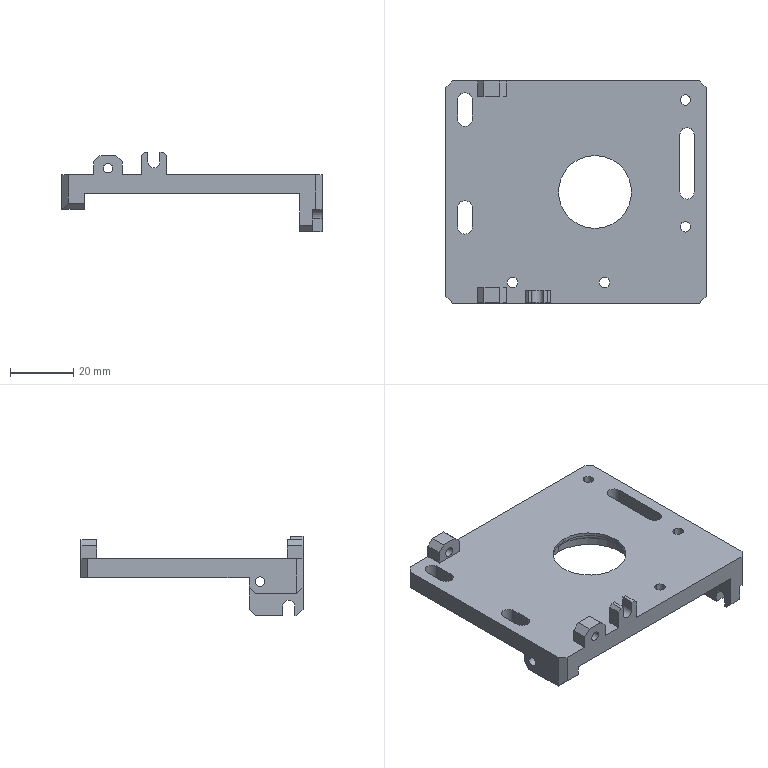NC program | NX | posted with a generic post | part box 82 x 70 x 25 mm
Lines 1409 to 2271 of 8354:
(ZLEVEL_PROFILE_1_1 , TOOL : D3)
N2792 T03 M6
N2794 G54
N2796 G17 G0 G90 X6.477 Y34.25 S9500 M3
N2798 G43 Z30. H3
N2800 Z-11.
N2802 G94 G1 X18.123 Z-11.61 F1000.
N2804 X18.342 Y34.321 Z-11.622
N2806 X18.541 Y34.466 Z-11.635
N2808 X18.704 Y34.713 Z-11.651
N2810 X18.76 Y35.005 Z-11.666
N2812 X18.7 Y35.295 Z-11.682
N2814 X18.534 Y35.541 Z-11.697
N2816 X18.333 Y35.683 Z-11.71
N2818 X18.123 Y35.75 Z-11.722
N2820 X9.001 Z-12.2
N2822 X0.001 F1300.
N2824 G3 X-0.75 Y35.008 R0.75
N2826 X0.007 Y34.25 R0.75
N2828 G1 X18.
N2830 G3 X18.75 Y35. R0.75
N2832 X18. Y35.75 R0.75
N2834 G1 X9.001
N2836 X0.224 Z-12.353
N2838 X0.102 Z-12.355
N2840 X-0.019 Y35.744 Z-12.357
N2842 X-0.186 Y35.718 Z-12.36
N2844 X-0.256 Y35.699 Z-12.362
N2846 X-0.381 Y35.639 Z-12.364
N2848 X-0.466 Y35.581 Z-12.366
N2850 X-0.532 Y35.517 Z-12.368
N2852 X-0.565 Y35.486
N2854 X-0.587 Y35.458 Z-12.369
N2856 X-0.625 Y35.4 Z-12.37
N2858 X-0.675 Y35.309 Z-12.372
N2860 X-0.697 Y35.263 Z-12.373
N2862 X-0.706 Y35.236
N2864 X-0.72 Y35.18 Z-12.374
N2866 X-0.743 Y35.02 Z-12.377
N2868 X-0.74 Y34.94 Z-12.379
N2870 X-0.714 Y34.797 Z-12.381
N2872 X-0.682 Y34.707 Z-12.383
N2874 X-0.611 Y34.58 Z-12.386
N2876 X-0.554 Y34.503 Z-12.387
N2878 X-0.458 Y34.414 Z-12.39
N2880 X-0.367 Y34.352 Z-12.391
N2882 X-0.236 Y34.288 Z-12.394
N2884 X-0.205 Y34.279 Z-12.395
N2886 X-0.142 Y34.264 Z-12.396
N2888 X-0.02 Y34.256 Z-12.398
N2890 X0.101 Y34.25 Z-12.4
N2892 X18.
N2894 G3 X18.75 Y35. R0.75
N2896 X18. Y35.75 R0.75
N2898 G1 X9.001
N2900 X0.224 Z-12.553
N2902 X0.102 Z-12.555
N2904 X-0.019 Y35.744 Z-12.557
N2906 X-0.186 Y35.718 Z-12.56
N2908 X-0.256 Y35.699 Z-12.562
N2910 X-0.381 Y35.639 Z-12.564
N2912 X-0.466 Y35.581 Z-12.566
N2914 X-0.532 Y35.517 Z-12.568
N2916 X-0.565 Y35.486
N2918 X-0.587 Y35.458 Z-12.569
N2920 X-0.625 Y35.4 Z-12.57
N2922 X-0.675 Y35.309 Z-12.572
N2924 X-0.697 Y35.263 Z-12.573
N2926 X-0.706 Y35.236
N2928 X-0.72 Y35.18 Z-12.574
N2930 X-0.743 Y35.02 Z-12.577
N2932 X-0.74 Y34.94 Z-12.579
N2934 X-0.714 Y34.797 Z-12.581
N2936 X-0.682 Y34.707 Z-12.583
N2938 X-0.611 Y34.58 Z-12.586
N2940 X-0.554 Y34.503 Z-12.587
N2942 X-0.458 Y34.414 Z-12.59
N2944 X-0.367 Y34.352 Z-12.591
N2946 X-0.236 Y34.288 Z-12.594
N2948 X-0.205 Y34.279 Z-12.595
N2950 X-0.142 Y34.264 Z-12.596
N2952 X-0.02 Y34.256 Z-12.598
N2954 X0.101 Y34.25 Z-12.6
N2956 X18.
N2958 G3 X18.75 Y35. R0.75
N2960 X18. Y35.75 R0.75
N2962 G1 X9.001
N2964 X0.224 Z-12.753
N2966 X0.102 Z-12.755
N2968 X-0.019 Y35.744 Z-12.757
N2970 X-0.186 Y35.718 Z-12.76
N2972 X-0.256 Y35.699 Z-12.762
N2974 X-0.381 Y35.639 Z-12.764
N2976 X-0.466 Y35.581 Z-12.766
N2978 X-0.532 Y35.517 Z-12.768
N2980 X-0.565 Y35.486
N2982 X-0.587 Y35.458 Z-12.769
N2984 X-0.625 Y35.4 Z-12.77
N2986 X-0.675 Y35.309 Z-12.772
N2988 X-0.697 Y35.263 Z-12.773
N2990 X-0.706 Y35.236
N2992 X-0.72 Y35.18 Z-12.774
N2994 X-0.743 Y35.02 Z-12.777
N2996 X-0.74 Y34.94 Z-12.779
N2998 X-0.714 Y34.797 Z-12.781
N3000 X-0.682 Y34.707 Z-12.783
N3002 X-0.611 Y34.58 Z-12.786
N3004 X-0.554 Y34.503 Z-12.787
N3006 X-0.458 Y34.414 Z-12.79
N3008 X-0.367 Y34.352 Z-12.791
N3010 X-0.236 Y34.288 Z-12.794
N3012 X-0.205 Y34.279 Z-12.795
N3014 X-0.142 Y34.264 Z-12.796
N3016 X-0.02 Y34.256 Z-12.798
N3018 X0.101 Y34.25 Z-12.8
N3020 X18.
N3022 G3 X18.75 Y35. R0.75
N3024 X18. Y35.75 R0.75
N3026 G1 X9.001
N3028 X0.224 Z-12.953
N3030 X0.102 Z-12.955
N3032 X-0.019 Y35.744 Z-12.957
N3034 X-0.186 Y35.718 Z-12.96
N3036 X-0.256 Y35.699 Z-12.962
N3038 X-0.381 Y35.639 Z-12.964
N3040 X-0.466 Y35.581 Z-12.966
N3042 X-0.532 Y35.517 Z-12.968
N3044 X-0.565 Y35.486
N3046 X-0.587 Y35.458 Z-12.969
N3048 X-0.625 Y35.4 Z-12.97
N3050 X-0.675 Y35.31 Z-12.972
N3052 X-0.697 Y35.263 Z-12.973
N3054 X-0.706 Y35.236
N3056 X-0.72 Y35.18 Z-12.974
N3058 X-0.743 Y35.021 Z-12.977
N3060 X-0.74 Y34.94 Z-12.979
N3062 X-0.714 Y34.797 Z-12.981
N3064 X-0.682 Y34.707 Z-12.983
N3066 X-0.611 Y34.58 Z-12.986
N3068 X-0.554 Y34.503 Z-12.987
N3070 X-0.458 Y34.414 Z-12.99
N3072 X-0.367 Y34.352 Z-12.991
N3074 X-0.236 Y34.288 Z-12.994
N3076 X-0.205 Y34.279 Z-12.995
N3078 X-0.142 Y34.264 Z-12.996
N3080 X-0.02 Y34.256 Z-12.998
N3082 X0.101 Y34.25 Z-13.
N3084 X18.
N3086 G3 X18.75 Y35. R0.75
N3088 X18. Y35.75 R0.75
N3090 G1 X9.001
N3092 X0.224 Z-13.153
N3094 X0.102 Z-13.155
N3096 X-0.019 Y35.744 Z-13.157
N3098 X-0.186 Y35.718 Z-13.16
N3100 X-0.256 Y35.699 Z-13.162
N3102 X-0.381 Y35.639 Z-13.164
N3104 X-0.466 Y35.581 Z-13.166
N3106 X-0.532 Y35.517 Z-13.168
N3108 X-0.565 Y35.486
N3110 X-0.587 Y35.458 Z-13.169
N3112 X-0.625 Y35.4 Z-13.17
N3114 X-0.675 Y35.31 Z-13.172
N3116 X-0.697 Y35.263 Z-13.173
N3118 X-0.706 Y35.236
N3120 X-0.72 Y35.18 Z-13.174
N3122 X-0.743 Y35.021 Z-13.177
N3124 X-0.74 Y34.94 Z-13.179
N3126 X-0.714 Y34.797 Z-13.181
N3128 X-0.682 Y34.707 Z-13.183
N3130 X-0.611 Y34.58 Z-13.186
N3132 X-0.554 Y34.503 Z-13.187
N3134 X-0.458 Y34.414 Z-13.19
N3136 X-0.367 Y34.352 Z-13.191
N3138 X-0.236 Y34.288 Z-13.194
N3140 X-0.205 Y34.279 Z-13.195
N3142 X-0.142 Y34.264 Z-13.196
N3144 X-0.02 Y34.256 Z-13.198
N3146 X0.101 Y34.25 Z-13.2
N3148 X18.
N3150 G3 X18.75 Y35. R0.75
N3152 X18. Y35.75 R0.75
N3154 G1 X9.001
N3156 X0.224 Z-13.353
N3158 X0.102 Z-13.355
N3160 X-0.019 Y35.744 Z-13.357
N3162 X-0.186 Y35.718 Z-13.36
N3164 X-0.256 Y35.699 Z-13.362
N3166 X-0.381 Y35.639 Z-13.364
N3168 X-0.466 Y35.581 Z-13.366
N3170 X-0.532 Y35.517 Z-13.368
N3172 X-0.565 Y35.486
N3174 X-0.587 Y35.458 Z-13.369
N3176 X-0.625 Y35.4 Z-13.37
N3178 X-0.675 Y35.31 Z-13.372
N3180 X-0.697 Y35.263 Z-13.373
N3182 X-0.706 Y35.236
N3184 X-0.72 Y35.18 Z-13.374
N3186 X-0.743 Y35.021 Z-13.377
N3188 X-0.74 Y34.94 Z-13.379
N3190 X-0.714 Y34.797 Z-13.381
N3192 X-0.682 Y34.707 Z-13.383
N3194 X-0.611 Y34.58 Z-13.386
N3196 X-0.554 Y34.503 Z-13.387
N3198 X-0.458 Y34.414 Z-13.39
N3200 X-0.367 Y34.352 Z-13.391
N3202 X-0.236 Y34.288 Z-13.394
N3204 X-0.205 Y34.279 Z-13.395
N3206 X-0.142 Y34.264 Z-13.396
N3208 X-0.02 Y34.256 Z-13.398
N3210 X0.101 Y34.25 Z-13.4
N3212 X18.
N3214 G3 X18.75 Y35. R0.75
N3216 X18. Y35.75 R0.75
N3218 G1 X9.001
N3220 X0.224 Z-13.553
N3222 X0.102 Z-13.555
N3224 X-0.019 Y35.744 Z-13.557
N3226 X-0.186 Y35.718 Z-13.56
N3228 X-0.256 Y35.699 Z-13.562
N3230 X-0.381 Y35.639 Z-13.564
N3232 X-0.466 Y35.581 Z-13.566
N3234 X-0.532 Y35.517 Z-13.568
N3236 X-0.565 Y35.486
N3238 X-0.587 Y35.458 Z-13.569
N3240 X-0.625 Y35.4 Z-13.57
N3242 X-0.675 Y35.31 Z-13.572
N3244 X-0.697 Y35.263 Z-13.573
N3246 X-0.706 Y35.236
N3248 X-0.72 Y35.18 Z-13.574
N3250 X-0.743 Y35.021 Z-13.577
N3252 X-0.74 Y34.94 Z-13.579
N3254 X-0.714 Y34.797 Z-13.581
N3256 X-0.682 Y34.707 Z-13.583
N3258 X-0.611 Y34.58 Z-13.586
N3260 X-0.554 Y34.503 Z-13.587
N3262 X-0.458 Y34.414 Z-13.59
N3264 X-0.367 Y34.352 Z-13.591
N3266 X-0.236 Y34.288 Z-13.594
N3268 X-0.205 Y34.279 Z-13.595
N3270 X-0.142 Y34.264 Z-13.596
N3272 X-0.02 Y34.256 Z-13.598
N3274 X0.101 Y34.25 Z-13.6
N3276 X18.
N3278 G3 X18.75 Y35. R0.75
N3280 X18. Y35.75 R0.75
N3282 G1 X9.001
N3284 X0.224 Z-13.753
N3286 X0.102 Z-13.755
N3288 X-0.019 Y35.744 Z-13.757
N3290 X-0.186 Y35.718 Z-13.76
N3292 X-0.256 Y35.699 Z-13.762
N3294 X-0.381 Y35.639 Z-13.764
N3296 X-0.466 Y35.581 Z-13.766
N3298 X-0.532 Y35.517 Z-13.768
N3300 X-0.565 Y35.486
N3302 X-0.587 Y35.458 Z-13.769
N3304 X-0.625 Y35.4 Z-13.77
N3306 X-0.675 Y35.31 Z-13.772
N3308 X-0.697 Y35.263 Z-13.773
N3310 X-0.706 Y35.236
N3312 X-0.72 Y35.18 Z-13.774
N3314 X-0.743 Y35.021 Z-13.777
N3316 X-0.74 Y34.94 Z-13.779
N3318 X-0.714 Y34.797 Z-13.781
N3320 X-0.682 Y34.707 Z-13.783
N3322 X-0.611 Y34.58 Z-13.786
N3324 X-0.554 Y34.503 Z-13.787
N3326 X-0.458 Y34.414 Z-13.79
N3328 X-0.367 Y34.352 Z-13.791
N3330 X-0.236 Y34.288 Z-13.794
N3332 X-0.205 Y34.279 Z-13.795
N3334 X-0.142 Y34.264 Z-13.796
N3336 X-0.02 Y34.256 Z-13.798
N3338 X0.101 Y34.25 Z-13.8
N3340 X18.
N3342 G3 X18.75 Y35. R0.75
N3344 X18. Y35.75 R0.75
N3346 G1 X9.001
N3348 X0.224 Z-13.953
N3350 X0.102 Z-13.955
N3352 X-0.019 Y35.744 Z-13.957
N3354 X-0.186 Y35.718 Z-13.96
N3356 X-0.256 Y35.699 Z-13.962
N3358 X-0.381 Y35.639 Z-13.964
N3360 X-0.466 Y35.581 Z-13.966
N3362 X-0.532 Y35.517 Z-13.968
N3364 X-0.565 Y35.486
N3366 X-0.587 Y35.458 Z-13.969
N3368 X-0.625 Y35.4 Z-13.97
N3370 X-0.675 Y35.31 Z-13.972
N3372 X-0.697 Y35.263 Z-13.973
N3374 X-0.706 Y35.236
N3376 X-0.72 Y35.18 Z-13.974
N3378 X-0.743 Y35.021 Z-13.977
N3380 X-0.74 Y34.94 Z-13.979
N3382 X-0.714 Y34.797 Z-13.981
N3384 X-0.682 Y34.707 Z-13.983
N3386 X-0.611 Y34.58 Z-13.986
N3388 X-0.554 Y34.503 Z-13.987
N3390 X-0.458 Y34.414 Z-13.99
N3392 X-0.367 Y34.352 Z-13.991
N3394 X-0.236 Y34.288 Z-13.994
N3396 X-0.205 Y34.279 Z-13.995
N3398 X-0.142 Y34.264 Z-13.996
N3400 X-0.02 Y34.256 Z-13.998
N3402 X0.101 Y34.25 Z-14.
N3404 X18.
N3406 G3 X18.75 Y35. R0.75
N3408 X18. Y35.75 R0.75
N3410 G1 X9.001
N3412 X0.224 Z-14.153
N3414 X0.102 Z-14.155
N3416 X-0.019 Y35.744 Z-14.157
N3418 X-0.186 Y35.718 Z-14.16
N3420 X-0.256 Y35.699 Z-14.162
N3422 X-0.381 Y35.639 Z-14.164
N3424 X-0.466 Y35.581 Z-14.166
N3426 X-0.532 Y35.517 Z-14.168
N3428 X-0.565 Y35.486
N3430 X-0.586 Y35.458 Z-14.169
N3432 X-0.625 Y35.4 Z-14.17
N3434 X-0.675 Y35.31 Z-14.172
N3436 X-0.697 Y35.263 Z-14.173
N3438 X-0.706 Y35.236
N3440 X-0.72 Y35.18 Z-14.174
N3442 X-0.743 Y35.021 Z-14.177
N3444 X-0.74 Y34.94 Z-14.179
N3446 X-0.714 Y34.797 Z-14.181
N3448 X-0.682 Y34.707 Z-14.183
N3450 X-0.611 Y34.58 Z-14.186
N3452 X-0.554 Y34.503 Z-14.187
N3454 X-0.458 Y34.414 Z-14.19
N3456 X-0.367 Y34.352 Z-14.191
N3458 X-0.236 Y34.288 Z-14.194
N3460 X-0.205 Y34.279 Z-14.195
N3462 X-0.142 Y34.264 Z-14.196
N3464 X-0.02 Y34.256 Z-14.198
N3466 X0.101 Y34.25 Z-14.2
N3468 X18.
N3470 G3 X18.75 Y35. R0.75
N3472 X18. Y35.75 R0.75
N3474 G1 X9.001
N3476 X0.224 Z-14.353
N3478 X0.102 Z-14.355
N3480 X-0.019 Y35.744 Z-14.357
N3482 X-0.186 Y35.718 Z-14.36
N3484 X-0.256 Y35.699 Z-14.362
N3486 X-0.381 Y35.639 Z-14.364
N3488 X-0.466 Y35.581 Z-14.366
N3490 X-0.532 Y35.517 Z-14.368
N3492 X-0.565 Y35.486
N3494 X-0.586 Y35.458 Z-14.369
N3496 X-0.625 Y35.4 Z-14.37
N3498 X-0.675 Y35.31 Z-14.372
N3500 X-0.697 Y35.263 Z-14.373
N3502 X-0.706 Y35.236
N3504 X-0.72 Y35.18 Z-14.374
N3506 X-0.743 Y35.021 Z-14.377
N3508 X-0.74 Y34.94 Z-14.379
N3510 X-0.714 Y34.797 Z-14.381
N3512 X-0.682 Y34.707 Z-14.383
N3514 X-0.611 Y34.58 Z-14.386
N3516 X-0.554 Y34.503 Z-14.387
N3518 X-0.458 Y34.414 Z-14.39
N3520 X-0.367 Y34.352 Z-14.391
N3522 X-0.236 Y34.288 Z-14.394
N3524 X-0.205 Y34.279 Z-14.395
N3526 X-0.142 Y34.264 Z-14.396
N3528 X-0.02 Y34.256 Z-14.398
N3530 X0.101 Y34.25 Z-14.4
N3532 X18.
N3534 G3 X18.75 Y35. R0.75
N3536 X18. Y35.75 R0.75
N3538 G1 X9.001
N3540 X0.224 Z-14.553
N3542 X0.102 Z-14.555
N3544 X-0.019 Y35.744 Z-14.557
N3546 X-0.186 Y35.718 Z-14.56
N3548 X-0.256 Y35.699 Z-14.562
N3550 X-0.381 Y35.639 Z-14.564
N3552 X-0.466 Y35.581 Z-14.566
N3554 X-0.532 Y35.517 Z-14.568
N3556 X-0.565 Y35.486
N3558 X-0.586 Y35.458 Z-14.569
N3560 X-0.625 Y35.4 Z-14.57
N3562 X-0.675 Y35.31 Z-14.572
N3564 X-0.697 Y35.263 Z-14.573
N3566 X-0.706 Y35.236
N3568 X-0.72 Y35.18 Z-14.574
N3570 X-0.743 Y35.021 Z-14.577
N3572 X-0.74 Y34.94 Z-14.579
N3574 X-0.714 Y34.797 Z-14.581
N3576 X-0.682 Y34.707 Z-14.583
N3578 X-0.611 Y34.58 Z-14.586
N3580 X-0.554 Y34.503 Z-14.587
N3582 X-0.458 Y34.414 Z-14.59
N3584 X-0.367 Y34.352 Z-14.591
N3586 X-0.236 Y34.288 Z-14.594
N3588 X-0.205 Y34.279 Z-14.595
N3590 X-0.142 Y34.264 Z-14.596
N3592 X-0.02 Y34.256 Z-14.598
N3594 X0.101 Y34.25 Z-14.6
N3596 X18.
N3598 G3 X18.75 Y35. R0.75
N3600 X18. Y35.75 R0.75
N3602 G1 X9.001
N3604 X0.224 Z-14.753
N3606 X0.102 Z-14.755
N3608 X-0.019 Y35.744 Z-14.757
N3610 X-0.186 Y35.718 Z-14.76
N3612 X-0.256 Y35.699 Z-14.762
N3614 X-0.381 Y35.639 Z-14.764
N3616 X-0.466 Y35.581 Z-14.766
N3618 X-0.532 Y35.517 Z-14.768
N3620 X-0.565 Y35.486
N3622 X-0.586 Y35.458 Z-14.769
N3624 X-0.625 Y35.4 Z-14.77
N3626 X-0.675 Y35.31 Z-14.772
N3628 X-0.697 Y35.263 Z-14.773
N3630 X-0.706 Y35.236
N3632 X-0.72 Y35.18 Z-14.774
N3634 X-0.743 Y35.021 Z-14.777
N3636 X-0.74 Y34.94 Z-14.779
N3638 X-0.714 Y34.797 Z-14.781
N3640 X-0.682 Y34.707 Z-14.783
N3642 X-0.611 Y34.58 Z-14.786
N3644 X-0.554 Y34.503 Z-14.787
N3646 X-0.458 Y34.414 Z-14.79
N3648 X-0.367 Y34.352 Z-14.791
N3650 X-0.236 Y34.288 Z-14.794
N3652 X-0.205 Y34.279 Z-14.795
N3654 X-0.142 Y34.264 Z-14.796
N3656 X-0.02 Y34.256 Z-14.798
N3658 X0.101 Y34.25 Z-14.8
N3660 X18.
N3662 G3 X18.75 Y35. R0.75
N3664 X18. Y35.75 R0.75
N3666 G1 X9.001
N3668 X0.224 Z-14.953
N3670 X0.102 Z-14.955
N3672 X-0.019 Y35.744 Z-14.957
N3674 X-0.186 Y35.718 Z-14.96
N3676 X-0.256 Y35.699 Z-14.962
N3678 X-0.381 Y35.639 Z-14.964
N3680 X-0.466 Y35.581 Z-14.966
N3682 X-0.532 Y35.517 Z-14.968
N3684 X-0.565 Y35.486
N3686 X-0.586 Y35.458 Z-14.969
N3688 X-0.625 Y35.4 Z-14.97
N3690 X-0.675 Y35.31 Z-14.972
N3692 X-0.697 Y35.263 Z-14.973
N3694 X-0.706 Y35.236
N3696 X-0.72 Y35.18 Z-14.974
N3698 X-0.743 Y35.021 Z-14.977
N3700 X-0.74 Y34.94 Z-14.979
N3702 X-0.714 Y34.797 Z-14.981
N3704 X-0.682 Y34.707 Z-14.983
N3706 X-0.611 Y34.58 Z-14.986
N3708 X-0.554 Y34.503 Z-14.987
N3710 X-0.458 Y34.414 Z-14.99
N3712 X-0.367 Y34.352 Z-14.991
N3714 X-0.236 Y34.288 Z-14.994
N3716 X-0.205 Y34.279 Z-14.995
N3718 X-0.142 Y34.264 Z-14.996
N3720 X-0.02 Y34.256 Z-14.998
N3722 X0.101 Y34.25 Z-15.
N3724 X18.
N3726 G3 X18.75 Y35. R0.75
N3728 X18. Y35.75 R0.75
N3730 G1 X9.001
N3732 X0.224 Z-15.153
N3734 X0.102 Z-15.155
N3736 X-0.019 Y35.744 Z-15.157
N3738 X-0.186 Y35.718 Z-15.16
N3740 X-0.256 Y35.699 Z-15.162
N3742 X-0.381 Y35.639 Z-15.164
N3744 X-0.466 Y35.581 Z-15.166
N3746 X-0.532 Y35.517 Z-15.168
N3748 X-0.565 Y35.486
N3750 X-0.586 Y35.458 Z-15.169
N3752 X-0.625 Y35.4 Z-15.17
N3754 X-0.675 Y35.31 Z-15.172
N3756 X-0.697 Y35.263 Z-15.173
N3758 X-0.706 Y35.236
N3760 X-0.72 Y35.18 Z-15.174
N3762 X-0.743 Y35.021 Z-15.177
N3764 X-0.74 Y34.94 Z-15.179
N3766 X-0.714 Y34.797 Z-15.181
N3768 X-0.682 Y34.707 Z-15.183
N3770 X-0.611 Y34.58 Z-15.186
N3772 X-0.554 Y34.503 Z-15.187
N3774 X-0.458 Y34.414 Z-15.19
N3776 X-0.367 Y34.352 Z-15.191
N3778 X-0.236 Y34.288 Z-15.194
N3780 X-0.205 Y34.279 Z-15.195
N3782 X-0.142 Y34.264 Z-15.196
N3784 X-0.02 Y34.256 Z-15.198
N3786 X0.101 Y34.25 Z-15.2
N3788 X18.
N3790 G3 X18.75 Y35. R0.75
N3792 X18. Y35.75 R0.75
N3794 G1 X9.001
N3796 X0.224 Z-15.353
N3798 X0.102 Z-15.355
N3800 X-0.019 Y35.744 Z-15.357
N3802 X-0.186 Y35.718 Z-15.36
N3804 X-0.256 Y35.699 Z-15.362
N3806 X-0.381 Y35.639 Z-15.364
N3808 X-0.466 Y35.581 Z-15.366
N3810 X-0.532 Y35.517 Z-15.368
N3812 X-0.565 Y35.486
N3814 X-0.586 Y35.458 Z-15.369
N3816 X-0.625 Y35.4 Z-15.37
N3818 X-0.675 Y35.31 Z-15.372
N3820 X-0.697 Y35.263 Z-15.373
N3822 X-0.706 Y35.236
N3824 X-0.72 Y35.18 Z-15.374
N3826 X-0.743 Y35.021 Z-15.377
N3828 X-0.74 Y34.94 Z-15.379
N3830 X-0.714 Y34.797 Z-15.381
N3832 X-0.682 Y34.707 Z-15.383
N3834 X-0.611 Y34.58 Z-15.386
N3836 X-0.554 Y34.503 Z-15.387
N3838 X-0.458 Y34.414 Z-15.39
N3840 X-0.367 Y34.352 Z-15.391
N3842 X-0.236 Y34.288 Z-15.394
N3844 X-0.205 Y34.279 Z-15.395
N3846 X-0.142 Y34.264 Z-15.396
N3848 X-0.02 Y34.256 Z-15.398
N3850 X0.101 Y34.25 Z-15.4
N3852 X18.
N3854 G3 X18.75 Y35. R0.75
N3856 X18. Y35.75 R0.75
N3858 G1 X9.001
N3860 X0.224 Z-15.553
N3862 X0.102 Z-15.555
N3864 X-0.019 Y35.744 Z-15.557
N3866 X-0.186 Y35.718 Z-15.56
N3868 X-0.256 Y35.699 Z-15.562
N3870 X-0.381 Y35.639 Z-15.564
N3872 X-0.466 Y35.581 Z-15.566
N3874 X-0.532 Y35.517 Z-15.568
N3876 X-0.565 Y35.486
N3878 X-0.586 Y35.458 Z-15.569
N3880 X-0.625 Y35.4 Z-15.57
N3882 X-0.675 Y35.31 Z-15.572
N3884 X-0.697 Y35.263 Z-15.573
N3886 X-0.706 Y35.236
N3888 X-0.72 Y35.18 Z-15.574
N3890 X-0.743 Y35.021 Z-15.577
N3892 X-0.74 Y34.94 Z-15.579
N3894 X-0.714 Y34.797 Z-15.581
N3896 X-0.682 Y34.707 Z-15.583
N3898 X-0.611 Y34.58 Z-15.586
N3900 X-0.554 Y34.503 Z-15.587
N3902 X-0.458 Y34.414 Z-15.59
N3904 X-0.367 Y34.352 Z-15.591
N3906 X-0.236 Y34.288 Z-15.594
N3908 X-0.205 Y34.279 Z-15.595
N3910 X-0.142 Y34.264 Z-15.596
N3912 X-0.02 Y34.256 Z-15.598
N3914 X0.101 Y34.25 Z-15.6
N3916 X18.
N3918 G3 X18.75 Y35. R0.75
N3920 X18. Y35.75 R0.75
N3922 G1 X9.001
N3924 X0.224 Z-15.753
N3926 X0.102 Z-15.755
N3928 X-0.019 Y35.744 Z-15.757
N3930 X-0.186 Y35.718 Z-15.76
N3932 X-0.256 Y35.699 Z-15.762
N3934 X-0.381 Y35.639 Z-15.764
N3936 X-0.466 Y35.581 Z-15.766
N3938 X-0.532 Y35.517 Z-15.768
N3940 X-0.565 Y35.486
N3942 X-0.586 Y35.458 Z-15.769
N3944 X-0.625 Y35.4 Z-15.77
N3946 X-0.675 Y35.31 Z-15.772
N3948 X-0.697 Y35.263 Z-15.773
N3950 X-0.706 Y35.236
N3952 X-0.72 Y35.18 Z-15.774
N3954 X-0.743 Y35.021 Z-15.777
N3956 X-0.74 Y34.94 Z-15.779
N3958 X-0.714 Y34.797 Z-15.781
N3960 X-0.682 Y34.707 Z-15.783
N3962 X-0.611 Y34.58 Z-15.786
N3964 X-0.554 Y34.503 Z-15.787
N3966 X-0.458 Y34.414 Z-15.79
N3968 X-0.367 Y34.352 Z-15.791
N3970 X-0.236 Y34.288 Z-15.794
N3972 X-0.205 Y34.279 Z-15.795
N3974 X-0.142 Y34.264 Z-15.796
N3976 X-0.02 Y34.256 Z-15.798
N3978 X0.101 Y34.25 Z-15.8
N3980 X18.
N3982 G3 X18.75 Y35. R0.75
N3984 X18. Y35.75 R0.75
N3986 G1 X9.001
N3988 X0.224 Z-15.953
N3990 X0.102 Z-15.955
N3992 X-0.019 Y35.744 Z-15.957
N3994 X-0.186 Y35.718 Z-15.96
N3996 X-0.256 Y35.699 Z-15.962
N3998 X-0.381 Y35.639 Z-15.964
N4000 X-0.466 Y35.581 Z-15.966
N4002 X-0.532 Y35.517 Z-15.968
N4004 X-0.565 Y35.486
N4006 X-0.586 Y35.458 Z-15.969
N4008 X-0.625 Y35.4 Z-15.97
N4010 X-0.675 Y35.31 Z-15.972
N4012 X-0.697 Y35.263 Z-15.973
N4014 X-0.706 Y35.236
N4016 X-0.72 Y35.18 Z-15.974
N4018 X-0.743 Y35.021 Z-15.977
N4020 X-0.74 Y34.94 Z-15.979
N4022 X-0.714 Y34.797 Z-15.981
N4024 X-0.682 Y34.707 Z-15.983
N4026 X-0.611 Y34.58 Z-15.986
N4028 X-0.554 Y34.503 Z-15.987
N4030 X-0.458 Y34.414 Z-15.99
N4032 X-0.367 Y34.352 Z-15.991
N4034 X-0.236 Y34.288 Z-15.994
N4036 X-0.205 Y34.279 Z-15.995
N4038 X-0.142 Y34.264 Z-15.996
N4040 X-0.02 Y34.256 Z-15.998
N4042 X0.101 Y34.25 Z-16.
N4044 X18.
N4046 G3 X18.75 Y35. R0.75
N4048 X18. Y35.75 R0.75
N4050 G1 X9.001
N4052 X0.224 Z-16.153
N4054 X0.102 Z-16.155
N4056 X-0.019 Y35.744 Z-16.157
N4058 X-0.186 Y35.718 Z-16.16
N4060 X-0.256 Y35.699 Z-16.162
N4062 X-0.381 Y35.639 Z-16.164
N4064 X-0.466 Y35.581 Z-16.166
N4066 X-0.532 Y35.517 Z-16.168
N4068 X-0.565 Y35.486
N4070 X-0.586 Y35.458 Z-16.169
N4072 X-0.625 Y35.4 Z-16.17
N4074 X-0.675 Y35.31 Z-16.172
N4076 X-0.697 Y35.263 Z-16.173
N4078 X-0.706 Y35.236
N4080 X-0.72 Y35.18 Z-16.174
N4082 X-0.743 Y35.021 Z-16.177
N4084 X-0.74 Y34.94 Z-16.179
N4086 X-0.714 Y34.797 Z-16.181
N4088 X-0.682 Y34.707 Z-16.183
N4090 X-0.611 Y34.58 Z-16.186
N4092 X-0.554 Y34.503 Z-16.187
N4094 X-0.458 Y34.414 Z-16.19
N4096 X-0.367 Y34.352 Z-16.191
N4098 X-0.236 Y34.288 Z-16.194
N4100 X-0.205 Y34.279 Z-16.195
N4102 X-0.142 Y34.264 Z-16.196
N4104 X-0.02 Y34.256 Z-16.198
N4106 X0.101 Y34.25 Z-16.2
N4108 X18.
N4110 G3 X18.75 Y35. R0.75
N4112 X18. Y35.75 R0.75
N4114 G1 X9.001
N4116 X0.224 Z-16.353
N4118 X0.102 Z-16.355
N4120 X-0.019 Y35.744 Z-16.357
N4122 X-0.186 Y35.718 Z-16.36
N4124 X-0.256 Y35.699 Z-16.362
N4126 X-0.381 Y35.639 Z-16.364
N4128 X-0.466 Y35.581 Z-16.366
N4130 X-0.532 Y35.517 Z-16.368
N4132 X-0.565 Y35.486
N4134 X-0.586 Y35.458 Z-16.369
N4136 X-0.625 Y35.4 Z-16.37
N4138 X-0.675 Y35.31 Z-16.372
N4140 X-0.697 Y35.263 Z-16.373
N4142 X-0.706 Y35.236
N4144 X-0.72 Y35.18 Z-16.374
N4146 X-0.743 Y35.021 Z-16.377
N4148 X-0.74 Y34.94 Z-16.379
N4150 X-0.714 Y34.797 Z-16.381
N4152 X-0.682 Y34.707 Z-16.383
N4154 X-0.611 Y34.58 Z-16.386
N4156 X-0.554 Y34.503 Z-16.387
N4158 X-0.458 Y34.414 Z-16.39
N4160 X-0.367 Y34.352 Z-16.391
N4162 X-0.236 Y34.288 Z-16.394
N4164 X-0.205 Y34.279 Z-16.395
N4166 X-0.142 Y34.264 Z-16.396
N4168 X-0.02 Y34.256 Z-16.398
N4170 X0.101 Y34.25 Z-16.4
N4172 X18.
N4174 G3 X18.75 Y35. R0.75
N4176 X18. Y35.75 R0.75
N4178 G1 X9.001
N4180 X0.224 Z-16.553
N4182 X0.102 Z-16.555
N4184 X-0.019 Y35.744 Z-16.557
N4186 X-0.186 Y35.718 Z-16.56
N4188 X-0.256 Y35.699 Z-16.562
N4190 X-0.381 Y35.639 Z-16.564
N4192 X-0.466 Y35.581 Z-16.566
N4194 X-0.532 Y35.517 Z-16.568
N4196 X-0.565 Y35.486
N4198 X-0.586 Y35.458 Z-16.569
N4200 X-0.625 Y35.4 Z-16.57
N4202 X-0.675 Y35.31 Z-16.572
N4204 X-0.697 Y35.263 Z-16.573
N4206 X-0.706 Y35.236
N4208 X-0.72 Y35.18 Z-16.574
N4210 X-0.743 Y35.021 Z-16.577
N4212 X-0.74 Y34.94 Z-16.579
N4214 X-0.714 Y34.797 Z-16.581
N4216 X-0.682 Y34.707 Z-16.583
N4218 X-0.611 Y34.58 Z-16.586
N4220 X-0.554 Y34.503 Z-16.587
N4222 X-0.458 Y34.414 Z-16.59
N4224 X-0.367 Y34.352 Z-16.591
N4226 X-0.236 Y34.288 Z-16.594
N4228 X-0.205 Y34.279 Z-16.595
N4230 X-0.142 Y34.264 Z-16.596
N4232 X-0.02 Y34.256 Z-16.598
N4234 X0.101 Y34.25 Z-16.6
N4236 X18.
N4238 G3 X18.75 Y35. R0.75
N4240 X18. Y35.75 R0.75
N4242 G1 X9.001
N4244 X0.224 Z-16.753
N4246 X0.102 Z-16.755
N4248 X-0.019 Y35.744 Z-16.757
N4250 X-0.186 Y35.718 Z-16.76
N4252 X-0.256 Y35.699 Z-16.762
N4254 X-0.381 Y35.639 Z-16.764
N4256 X-0.466 Y35.581 Z-16.766
N4258 X-0.532 Y35.517 Z-16.768
N4260 X-0.565 Y35.486
N4262 X-0.586 Y35.458 Z-16.769
N4264 X-0.625 Y35.4 Z-16.77
N4266 X-0.675 Y35.31 Z-16.772
N4268 X-0.697 Y35.263 Z-16.773
N4270 X-0.706 Y35.236
N4272 X-0.72 Y35.18 Z-16.774
N4274 X-0.743 Y35.021 Z-16.777
N4276 X-0.74 Y34.94 Z-16.779
N4278 X-0.714 Y34.797 Z-16.781
N4280 X-0.682 Y34.707 Z-16.783
N4282 X-0.611 Y34.58 Z-16.786
N4284 X-0.554 Y34.503 Z-16.787
N4286 X-0.458 Y34.414 Z-16.79
N4288 X-0.367 Y34.352 Z-16.791
N4290 X-0.236 Y34.288 Z-16.794
N4292 X-0.205 Y34.279 Z-16.795
N4294 X-0.142 Y34.264 Z-16.796
N4296 X-0.02 Y34.256 Z-16.798
N4298 X0.101 Y34.25 Z-16.8
N4300 X18.
N4302 G3 X18.75 Y35. R0.75
N4304 X18. Y35.75 R0.75
N4306 G1 X9.001
N4308 X0.224 Z-16.953
N4310 X0.102 Z-16.955
N4312 X-0.019 Y35.744 Z-16.957
N4314 X-0.186 Y35.718 Z-16.96
N4316 X-0.256 Y35.699 Z-16.962
N4318 X-0.381 Y35.639 Z-16.964
N4320 X-0.466 Y35.581 Z-16.966
N4322 X-0.532 Y35.517 Z-16.968
N4324 X-0.565 Y35.486
N4326 X-0.586 Y35.458 Z-16.969
N4328 X-0.625 Y35.4 Z-16.97
N4330 X-0.675 Y35.31 Z-16.972
N4332 X-0.697 Y35.263 Z-16.973
N4334 X-0.706 Y35.236
N4336 X-0.72 Y35.18 Z-16.974
N4338 X-0.743 Y35.021 Z-16.977
N4340 X-0.74 Y34.94 Z-16.979
N4342 X-0.714 Y34.797 Z-16.981
N4344 X-0.682 Y34.707 Z-16.983
N4346 X-0.611 Y34.58 Z-16.986
N4348 X-0.554 Y34.503 Z-16.987
N4350 X-0.458 Y34.414 Z-16.99
N4352 X-0.367 Y34.352 Z-16.991
N4354 X-0.236 Y34.288 Z-16.994
N4356 X-0.205 Y34.279 Z-16.995
N4358 X-0.142 Y34.264 Z-16.996
N4360 X-0.02 Y34.256 Z-16.998
N4362 X0.101 Y34.25 Z-17.
N4364 X18.
N4366 G3 X18.75 Y35. R0.75
N4368 X18. Y35.75 R0.75
N4370 G1 X9.001
N4372 X0.224 Z-17.153
N4374 X0.102 Z-17.155
N4376 X-0.019 Y35.744 Z-17.157
N4378 X-0.186 Y35.718 Z-17.16
N4380 X-0.256 Y35.699 Z-17.162
N4382 X-0.381 Y35.639 Z-17.164
N4384 X-0.466 Y35.581 Z-17.166
N4386 X-0.532 Y35.517 Z-17.168
N4388 X-0.565 Y35.486
N4390 X-0.586 Y35.458 Z-17.169
N4392 X-0.625 Y35.4 Z-17.17
N4394 X-0.675 Y35.31 Z-17.172
N4396 X-0.697 Y35.263 Z-17.173
N4398 X-0.706 Y35.236
N4400 X-0.72 Y35.18 Z-17.174
N4402 X-0.743 Y35.021 Z-17.177
N4404 X-0.74 Y34.94 Z-17.179
N4406 X-0.714 Y34.797 Z-17.181
N4408 X-0.682 Y34.707 Z-17.183
N4410 X-0.611 Y34.58 Z-17.186
N4412 X-0.554 Y34.503 Z-17.187
N4414 X-0.458 Y34.414 Z-17.19
N4416 X-0.367 Y34.352 Z-17.191
N4418 X-0.236 Y34.288 Z-17.194
N4420 X-0.205 Y34.279 Z-17.195
N4422 X-0.142 Y34.264 Z-17.196
N4424 X-0.02 Y34.256 Z-17.198
N4426 X0.101 Y34.25 Z-17.2
N4428 X18.
N4430 G3 X18.75 Y35. R0.75
N4432 X18. Y35.75 R0.75
N4434 G1 X9.001
N4436 X0.224 Z-17.353
N4438 X0.102 Z-17.355
N4440 X-0.019 Y35.744 Z-17.357
N4442 X-0.186 Y35.718 Z-17.36
N4444 X-0.256 Y35.699 Z-17.362
N4446 X-0.381 Y35.639 Z-17.364
N4448 X-0.466 Y35.581 Z-17.366
N4450 X-0.532 Y35.517 Z-17.368
N4452 X-0.565 Y35.486
N4454 X-0.586 Y35.458 Z-17.369
N4456 X-0.625 Y35.4 Z-17.37
N4458 X-0.675 Y35.31 Z-17.372
N4460 X-0.697 Y35.263 Z-17.373
N4462 X-0.706 Y35.236
N4464 X-0.72 Y35.18 Z-17.374
N4466 X-0.743 Y35.021 Z-17.377
N4468 X-0.74 Y34.94 Z-17.379
N4470 X-0.714 Y34.797 Z-17.381
N4472 X-0.682 Y34.707 Z-17.383
N4474 X-0.611 Y34.58 Z-17.386
N4476 X-0.554 Y34.503 Z-17.387
N4478 X-0.458 Y34.414 Z-17.39
N4480 X-0.367 Y34.352 Z-17.391
N4482 X-0.236 Y34.288 Z-17.394
N4484 X-0.205 Y34.279 Z-17.395
N4486 X-0.142 Y34.264 Z-17.396
N4488 X-0.02 Y34.256 Z-17.398
N4490 X0.101 Y34.25 Z-17.4
N4492 X18.
N4494 G3 X18.75 Y35. R0.75
N4496 X18. Y35.75 R0.75
N4498 G1 X9.001
N4500 X0.224 Z-17.553
N4502 X0.102 Z-17.555
N4504 X-0.019 Y35.744 Z-17.557
N4506 X-0.186 Y35.718 Z-17.56
N4508 X-0.256 Y35.699 Z-17.562
N4510 X-0.381 Y35.639 Z-17.564